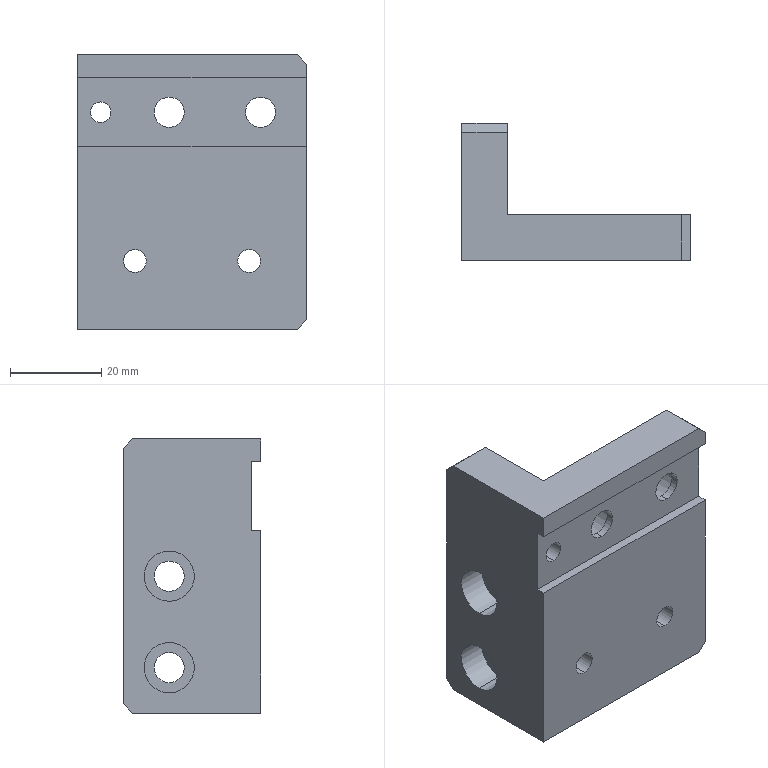Part | SolidWorks | features HoleWzd 4, Chamfer 1, Extrusion 1, ICE 1 | 1 solid | 45 faces | box 50 x 30 x 60 mm | volume 36632 mm3 | cylinder 24 | plane 21 | commonest cylinder face diameters 6.6 x8 11 x8 5 x4 4.5 x2 8 x2
STEP:
#1=CARTESIAN_POINT('',(12.5,10.,17.4));
#2=VERTEX_POINT('',#1);
#3=CARTESIAN_POINT('',(10.,10.,14.9));
#4=VERTEX_POINT('',#3);
#5=CARTESIAN_POINT('',(12.5,10.,14.9));
#6=DIRECTION('',(0.,-1.,0.));
#7=DIRECTION('',(0.,0.,-1.));
#8=AXIS2_PLACEMENT_3D('',#5,#6,#7);
#9=CIRCLE('',#8,2.5);
#10=EDGE_CURVE('',#2,#4,#9,.T.);
#11=ORIENTED_EDGE('',*,*,#10,.F.);
#12=CARTESIAN_POINT('',(12.5,0.,17.4));
#13=VERTEX_POINT('',#12);
#14=CARTESIAN_POINT('',(12.5,0.,17.4));
#15=DIRECTION('',(0.,-1.,0.));
#16=VECTOR('',#15,1000.);
#17=LINE('',#14,#16);
#18=EDGE_CURVE('',#2,#13,#17,.T.);
#19=ORIENTED_EDGE('',*,*,#18,.T.);
#20=CARTESIAN_POINT('',(12.5,0.,12.4));
#21=VERTEX_POINT('',#20);
#22=CARTESIAN_POINT('',(12.5,0.,14.9));
#23=DIRECTION('',(0.,-1.,0.));
#24=DIRECTION('',(0.,0.,-1.));
#25=AXIS2_PLACEMENT_3D('',#22,#23,#24);
#26=CIRCLE('',#25,2.5);
#27=EDGE_CURVE('',#13,#21,#26,.T.);
#28=ORIENTED_EDGE('',*,*,#27,.T.);
#29=CARTESIAN_POINT('',(12.5,10.,12.4));
#30=VERTEX_POINT('',#29);
#31=CARTESIAN_POINT('',(12.5,0.,12.4));
#32=DIRECTION('',(0.,-1.,0.));
#33=VECTOR('',#32,1000.);
#34=LINE('',#31,#33);
#35=EDGE_CURVE('',#30,#21,#34,.T.);
#36=ORIENTED_EDGE('',*,*,#35,.F.);
#37=CARTESIAN_POINT('',(12.5,10.,14.9));
#38=DIRECTION('',(0.,-1.,0.));
#39=DIRECTION('',(0.,0.,-1.));
#40=AXIS2_PLACEMENT_3D('',#37,#38,#39);
#41=CIRCLE('',#40,2.5);
#42=EDGE_CURVE('',#4,#30,#41,.T.);
#43=ORIENTED_EDGE('',*,*,#42,.F.);
#44=EDGE_LOOP('',(#11,#19,#28,#36,#43));
#45=FACE_OUTER_BOUND('',#44,.T.);
#46=CARTESIAN_POINT('',(12.5,0.,14.9));
#47=DIRECTION('',(0.,-1.,0.));
#48=DIRECTION('',(0.,0.,-1.));
#49=AXIS2_PLACEMENT_3D('',#46,#47,#48);
#50=CYLINDRICAL_SURFACE('',#49,2.5);
#51=ADVANCED_FACE('',(#45),#50,.F.);
#52=CARTESIAN_POINT('',(37.5,10.,17.4));
#53=VERTEX_POINT('',#52);
#54=CARTESIAN_POINT('',(37.5,10.,12.4));
#55=VERTEX_POINT('',#54);
#56=CARTESIAN_POINT('',(37.5,10.,14.9));
#57=DIRECTION('',(0.,-1.,0.));
#58=DIRECTION('',(0.,0.,-1.));
#59=AXIS2_PLACEMENT_3D('',#56,#57,#58);
#60=CIRCLE('',#59,2.5);
#61=EDGE_CURVE('',#53,#55,#60,.T.);
#62=ORIENTED_EDGE('',*,*,#61,.F.);
#63=CARTESIAN_POINT('',(37.5,0.,17.4));
#64=VERTEX_POINT('',#63);
#65=CARTESIAN_POINT('',(37.5,0.,17.4));
#66=DIRECTION('',(0.,-1.,0.));
#67=VECTOR('',#66,1000.);
#68=LINE('',#65,#67);
#69=EDGE_CURVE('',#53,#64,#68,.T.);
#70=ORIENTED_EDGE('',*,*,#69,.T.);
#71=CARTESIAN_POINT('',(37.5,0.,12.4));
#72=VERTEX_POINT('',#71);
#73=CARTESIAN_POINT('',(37.5,0.,14.9));
#74=DIRECTION('',(0.,-1.,0.));
#75=DIRECTION('',(0.,0.,-1.));
#76=AXIS2_PLACEMENT_3D('',#73,#74,#75);
#77=CIRCLE('',#76,2.5);
#78=EDGE_CURVE('',#64,#72,#77,.T.);
#79=ORIENTED_EDGE('',*,*,#78,.T.);
#80=CARTESIAN_POINT('',(37.5,0.,12.4));
#81=DIRECTION('',(0.,-1.,0.));
#82=VECTOR('',#81,1000.);
#83=LINE('',#80,#82);
#84=EDGE_CURVE('',#55,#72,#83,.T.);
#85=ORIENTED_EDGE('',*,*,#84,.F.);
#86=EDGE_LOOP('',(#62,#70,#79,#85));
#87=FACE_OUTER_BOUND('',#86,.T.);
#88=CARTESIAN_POINT('',(37.5,0.,14.9));
#89=DIRECTION('',(0.,-1.,0.));
#90=DIRECTION('',(0.,0.,-1.));
#91=AXIS2_PLACEMENT_3D('',#88,#89,#90);
#92=CYLINDRICAL_SURFACE('',#91,2.5);
#93=ADVANCED_FACE('',(#87),#92,.F.);
#94=CARTESIAN_POINT('',(6.4,20.,4.45));
#95=VERTEX_POINT('',#94);
#96=CARTESIAN_POINT('',(6.4,20.,15.45));
#97=VERTEX_POINT('',#96);
#98=CARTESIAN_POINT('',(6.4,20.,9.95));
#99=DIRECTION('',(-1.,0.,0.));
#100=DIRECTION('',(0.,0.,1.));
#101=AXIS2_PLACEMENT_3D('',#98,#99,#100);
#102=CIRCLE('',#101,5.5);
#103=EDGE_CURVE('',#95,#97,#102,.T.);
#104=ORIENTED_EDGE('',*,*,#103,.F.);
#105=CARTESIAN_POINT('',(0.,20.,4.45));
#106=VERTEX_POINT('',#105);
#107=CARTESIAN_POINT('',(0.,20.,4.45));
#108=DIRECTION('',(-1.,0.,0.));
#109=VECTOR('',#108,1000.);
#110=LINE('',#107,#109);
#111=EDGE_CURVE('',#95,#106,#110,.T.);
#112=ORIENTED_EDGE('',*,*,#111,.T.);
#113=CARTESIAN_POINT('',(0.,20.,15.45));
#114=VERTEX_POINT('',#113);
#115=CARTESIAN_POINT('',(0.,20.,9.95));
#116=DIRECTION('',(-1.,0.,0.));
#117=DIRECTION('',(0.,0.,1.));
#118=AXIS2_PLACEMENT_3D('',#115,#116,#117);
#119=CIRCLE('',#118,5.5);
#120=EDGE_CURVE('',#106,#114,#119,.T.);
#121=ORIENTED_EDGE('',*,*,#120,.T.);
#122=CARTESIAN_POINT('',(0.,20.,15.45));
#123=DIRECTION('',(-1.,0.,0.));
#124=VECTOR('',#123,1000.);
#125=LINE('',#122,#124);
#126=EDGE_CURVE('',#97,#114,#125,.T.);
#127=ORIENTED_EDGE('',*,*,#126,.F.);
#128=EDGE_LOOP('',(#104,#112,#121,#127));
#129=FACE_OUTER_BOUND('',#128,.T.);
#130=CARTESIAN_POINT('',(0.,20.,9.95));
#131=DIRECTION('',(-1.,0.,0.));
#132=DIRECTION('',(0.,0.,1.));
#133=AXIS2_PLACEMENT_3D('',#130,#131,#132);
#134=CYLINDRICAL_SURFACE('',#133,5.5);
#135=ADVANCED_FACE('',(#129),#134,.F.);
#136=CARTESIAN_POINT('',(10.,20.,6.65));
#137=VERTEX_POINT('',#136);
#138=CARTESIAN_POINT('',(10.,20.,13.25));
#139=VERTEX_POINT('',#138);
#140=CARTESIAN_POINT('',(10.,20.,9.95));
#141=DIRECTION('',(-1.,0.,0.));
#142=DIRECTION('',(0.,0.,1.));
#143=AXIS2_PLACEMENT_3D('',#140,#141,#142);
#144=CIRCLE('',#143,3.3);
#145=EDGE_CURVE('',#137,#139,#144,.T.);
#146=ORIENTED_EDGE('',*,*,#145,.F.);
#147=CARTESIAN_POINT('',(6.4,20.,6.65));
#148=VERTEX_POINT('',#147);
#149=CARTESIAN_POINT('',(0.,20.,6.65));
#150=DIRECTION('',(-1.,0.,0.));
#151=VECTOR('',#150,1000.);
#152=LINE('',#149,#151);
#153=EDGE_CURVE('',#137,#148,#152,.T.);
#154=ORIENTED_EDGE('',*,*,#153,.T.);
#155=CARTESIAN_POINT('',(6.4,20.,13.25));
#156=VERTEX_POINT('',#155);
#157=CARTESIAN_POINT('',(6.4,20.,9.95));
#158=DIRECTION('',(-1.,0.,0.));
#159=DIRECTION('',(0.,0.,1.));
#160=AXIS2_PLACEMENT_3D('',#157,#158,#159);
#161=CIRCLE('',#160,3.3);
#162=EDGE_CURVE('',#148,#156,#161,.T.);
#163=ORIENTED_EDGE('',*,*,#162,.T.);
#164=CARTESIAN_POINT('',(0.,20.,13.25));
#165=DIRECTION('',(-1.,0.,0.));
#166=VECTOR('',#165,1000.);
#167=LINE('',#164,#166);
#168=EDGE_CURVE('',#139,#156,#167,.T.);
#169=ORIENTED_EDGE('',*,*,#168,.F.);
#170=EDGE_LOOP('',(#146,#154,#163,#169));
#171=FACE_OUTER_BOUND('',#170,.T.);
#172=CARTESIAN_POINT('',(0.,20.,9.95));
#173=DIRECTION('',(-1.,0.,0.));
#174=DIRECTION('',(0.,0.,1.));
#175=AXIS2_PLACEMENT_3D('',#172,#173,#174);
#176=CYLINDRICAL_SURFACE('',#175,3.3);
#177=ADVANCED_FACE('',(#171),#176,.F.);
#178=CARTESIAN_POINT('',(6.4,20.,24.45));
#179=VERTEX_POINT('',#178);
#180=CARTESIAN_POINT('',(6.4,20.,35.45));
#181=VERTEX_POINT('',#180);
#182=CARTESIAN_POINT('',(6.4,20.,29.95));
#183=DIRECTION('',(-1.,0.,0.));
#184=DIRECTION('',(0.,0.,1.));
#185=AXIS2_PLACEMENT_3D('',#182,#183,#184);
#186=CIRCLE('',#185,5.5);
#187=EDGE_CURVE('',#179,#181,#186,.T.);
#188=ORIENTED_EDGE('',*,*,#187,.F.);
#189=CARTESIAN_POINT('',(0.,20.,24.45));
#190=VERTEX_POINT('',#189);
#191=CARTESIAN_POINT('',(0.,20.,24.45));
#192=DIRECTION('',(-1.,0.,0.));
#193=VECTOR('',#192,1000.);
#194=LINE('',#191,#193);
#195=EDGE_CURVE('',#179,#190,#194,.T.);
#196=ORIENTED_EDGE('',*,*,#195,.T.);
#197=CARTESIAN_POINT('',(0.,20.,35.45));
#198=VERTEX_POINT('',#197);
#199=CARTESIAN_POINT('',(0.,20.,29.95));
#200=DIRECTION('',(-1.,0.,0.));
#201=DIRECTION('',(0.,0.,1.));
#202=AXIS2_PLACEMENT_3D('',#199,#200,#201);
#203=CIRCLE('',#202,5.5);
#204=EDGE_CURVE('',#190,#198,#203,.T.);
#205=ORIENTED_EDGE('',*,*,#204,.T.);
#206=CARTESIAN_POINT('',(0.,20.,35.45));
#207=DIRECTION('',(-1.,0.,0.));
#208=VECTOR('',#207,1000.);
#209=LINE('',#206,#208);
#210=EDGE_CURVE('',#181,#198,#209,.T.);
#211=ORIENTED_EDGE('',*,*,#210,.F.);
#212=EDGE_LOOP('',(#188,#196,#205,#211));
#213=FACE_OUTER_BOUND('',#212,.T.);
#214=CARTESIAN_POINT('',(0.,20.,29.95));
#215=DIRECTION('',(-1.,0.,0.));
#216=DIRECTION('',(0.,0.,1.));
#217=AXIS2_PLACEMENT_3D('',#214,#215,#216);
#218=CYLINDRICAL_SURFACE('',#217,5.5);
#219=ADVANCED_FACE('',(#213),#218,.F.);
#220=CARTESIAN_POINT('',(10.,20.,26.65));
#221=VERTEX_POINT('',#220);
#222=CARTESIAN_POINT('',(10.,20.,33.25));
#223=VERTEX_POINT('',#222);
#224=CARTESIAN_POINT('',(10.,20.,29.95));
#225=DIRECTION('',(-1.,0.,0.));
#226=DIRECTION('',(0.,0.,1.));
#227=AXIS2_PLACEMENT_3D('',#224,#225,#226);
#228=CIRCLE('',#227,3.3);
#229=EDGE_CURVE('',#221,#223,#228,.T.);
#230=ORIENTED_EDGE('',*,*,#229,.F.);
#231=CARTESIAN_POINT('',(6.4,20.,26.65));
#232=VERTEX_POINT('',#231);
#233=CARTESIAN_POINT('',(0.,20.,26.65));
#234=DIRECTION('',(-1.,0.,0.));
#235=VECTOR('',#234,1000.);
#236=LINE('',#233,#235);
#237=EDGE_CURVE('',#221,#232,#236,.T.);
#238=ORIENTED_EDGE('',*,*,#237,.T.);
#239=CARTESIAN_POINT('',(6.4,20.,33.25));
#240=VERTEX_POINT('',#239);
#241=CARTESIAN_POINT('',(6.4,20.,29.95));
#242=DIRECTION('',(-1.,0.,0.));
#243=DIRECTION('',(0.,0.,1.));
#244=AXIS2_PLACEMENT_3D('',#241,#242,#243);
#245=CIRCLE('',#244,3.3);
#246=EDGE_CURVE('',#232,#240,#245,.T.);
#247=ORIENTED_EDGE('',*,*,#246,.T.);
#248=CARTESIAN_POINT('',(0.,20.,33.25));
#249=DIRECTION('',(-1.,0.,0.));
#250=VECTOR('',#249,1000.);
#251=LINE('',#248,#250);
#252=EDGE_CURVE('',#223,#240,#251,.T.);
#253=ORIENTED_EDGE('',*,*,#252,.F.);
#254=EDGE_LOOP('',(#230,#238,#247,#253));
#255=FACE_OUTER_BOUND('',#254,.T.);
#256=CARTESIAN_POINT('',(0.,20.,29.95));
#257=DIRECTION('',(-1.,0.,0.));
#258=DIRECTION('',(0.,0.,1.));
#259=AXIS2_PLACEMENT_3D('',#256,#257,#258);
#260=CYLINDRICAL_SURFACE('',#259,3.3);
#261=ADVANCED_FACE('',(#255),#260,.F.);
#262=CARTESIAN_POINT('',(20.,3.6,41.95));
#263=VERTEX_POINT('',#262);
#264=CARTESIAN_POINT('',(20.,3.6,52.95));
#265=VERTEX_POINT('',#264);
#266=CARTESIAN_POINT('',(20.,3.6,47.45));
#267=DIRECTION('',(0.,1.,0.));
#268=DIRECTION('',(0.,0.,1.));
#269=AXIS2_PLACEMENT_3D('',#266,#267,#268);
#270=CIRCLE('',#269,5.5);
#271=EDGE_CURVE('',#263,#265,#270,.T.);
#272=ORIENTED_EDGE('',*,*,#271,.F.);
#273=CARTESIAN_POINT('',(20.,10.,41.95));
#274=VERTEX_POINT('',#273);
#275=CARTESIAN_POINT('',(20.,10.,41.95));
#276=DIRECTION('',(0.,1.,0.));
#277=VECTOR('',#276,1000.);
#278=LINE('',#275,#277);
#279=EDGE_CURVE('',#263,#274,#278,.T.);
#280=ORIENTED_EDGE('',*,*,#279,.T.);
#281=CARTESIAN_POINT('',(20.,10.,52.95));
#282=VERTEX_POINT('',#281);
#283=CARTESIAN_POINT('',(20.,10.,47.45));
#284=DIRECTION('',(0.,1.,0.));
#285=DIRECTION('',(0.,0.,1.));
#286=AXIS2_PLACEMENT_3D('',#283,#284,#285);
#287=CIRCLE('',#286,5.5);
#288=EDGE_CURVE('',#274,#282,#287,.T.);
#289=ORIENTED_EDGE('',*,*,#288,.T.);
#290=CARTESIAN_POINT('',(20.,10.,52.95));
#291=DIRECTION('',(0.,1.,0.));
#292=VECTOR('',#291,1000.);
#293=LINE('',#290,#292);
#294=EDGE_CURVE('',#265,#282,#293,.T.);
#295=ORIENTED_EDGE('',*,*,#294,.F.);
#296=EDGE_LOOP('',(#272,#280,#289,#295));
#297=FACE_OUTER_BOUND('',#296,.T.);
#298=CARTESIAN_POINT('',(20.,10.,47.45));
#299=DIRECTION('',(0.,1.,0.));
#300=DIRECTION('',(0.,0.,1.));
#301=AXIS2_PLACEMENT_3D('',#298,#299,#300);
#302=CYLINDRICAL_SURFACE('',#301,5.5);
#303=ADVANCED_FACE('',(#297),#302,.F.);
#304=CARTESIAN_POINT('',(20.,2.,50.75));
#305=VERTEX_POINT('',#304);
#306=CARTESIAN_POINT('',(20.,2.,44.15));
#307=VERTEX_POINT('',#306);
#308=CARTESIAN_POINT('',(20.,2.,47.45));
#309=DIRECTION('',(0.,-1.,0.));
#310=DIRECTION('',(1.,0.,0.));
#311=AXIS2_PLACEMENT_3D('',#308,#309,#310);
#312=CIRCLE('',#311,3.3);
#313=EDGE_CURVE('',#305,#307,#312,.T.);
#314=ORIENTED_EDGE('',*,*,#313,.T.);
#315=CARTESIAN_POINT('',(20.,3.6,44.15));
#316=VERTEX_POINT('',#315);
#317=CARTESIAN_POINT('',(20.,10.,44.15));
#318=DIRECTION('',(0.,1.,0.));
#319=VECTOR('',#318,1000.);
#320=LINE('',#317,#319);
#321=EDGE_CURVE('',#307,#316,#320,.T.);
#322=ORIENTED_EDGE('',*,*,#321,.T.);
#323=CARTESIAN_POINT('',(20.,3.6,50.75));
#324=VERTEX_POINT('',#323);
#325=CARTESIAN_POINT('',(20.,3.6,47.45));
#326=DIRECTION('',(0.,1.,0.));
#327=DIRECTION('',(0.,0.,1.));
#328=AXIS2_PLACEMENT_3D('',#325,#326,#327);
#329=CIRCLE('',#328,3.3);
#330=EDGE_CURVE('',#316,#324,#329,.T.);
#331=ORIENTED_EDGE('',*,*,#330,.T.);
#332=CARTESIAN_POINT('',(20.,10.,50.75));
#333=DIRECTION('',(0.,1.,0.));
#334=VECTOR('',#333,1000.);
#335=LINE('',#332,#334);
#336=EDGE_CURVE('',#305,#324,#335,.T.);
#337=ORIENTED_EDGE('',*,*,#336,.F.);
#338=EDGE_LOOP('',(#314,#322,#331,#337));
#339=FACE_OUTER_BOUND('',#338,.T.);
#340=CARTESIAN_POINT('',(20.,10.,47.45));
#341=DIRECTION('',(0.,1.,0.));
#342=DIRECTION('',(0.,0.,1.));
#343=AXIS2_PLACEMENT_3D('',#340,#341,#342);
#344=CYLINDRICAL_SURFACE('',#343,3.3);
#345=ADVANCED_FACE('',(#339),#344,.F.);
#346=CARTESIAN_POINT('',(40.,3.6,41.95));
#347=VERTEX_POINT('',#346);
#348=CARTESIAN_POINT('',(40.,3.6,52.95));
#349=VERTEX_POINT('',#348);
#350=CARTESIAN_POINT('',(40.,3.6,47.45));
#351=DIRECTION('',(0.,1.,0.));
#352=DIRECTION('',(0.,0.,1.));
#353=AXIS2_PLACEMENT_3D('',#350,#351,#352);
#354=CIRCLE('',#353,5.5);
#355=EDGE_CURVE('',#347,#349,#354,.T.);
#356=ORIENTED_EDGE('',*,*,#355,.F.);
#357=CARTESIAN_POINT('',(40.,10.,41.95));
#358=VERTEX_POINT('',#357);
#359=CARTESIAN_POINT('',(40.,10.,41.95));
#360=DIRECTION('',(0.,1.,0.));
#361=VECTOR('',#360,1000.);
#362=LINE('',#359,#361);
#363=EDGE_CURVE('',#347,#358,#362,.T.);
#364=ORIENTED_EDGE('',*,*,#363,.T.);
#365=CARTESIAN_POINT('',(40.,10.,52.95));
#366=VERTEX_POINT('',#365);
#367=CARTESIAN_POINT('',(40.,10.,47.45));
#368=DIRECTION('',(0.,1.,0.));
#369=DIRECTION('',(0.,0.,1.));
#370=AXIS2_PLACEMENT_3D('',#367,#368,#369);
#371=CIRCLE('',#370,5.5);
#372=EDGE_CURVE('',#358,#366,#371,.T.);
#373=ORIENTED_EDGE('',*,*,#372,.T.);
#374=CARTESIAN_POINT('',(40.,10.,52.95));
#375=DIRECTION('',(0.,1.,0.));
#376=VECTOR('',#375,1000.);
#377=LINE('',#374,#376);
#378=EDGE_CURVE('',#349,#366,#377,.T.);
#379=ORIENTED_EDGE('',*,*,#378,.F.);
#380=EDGE_LOOP('',(#356,#364,#373,#379));
#381=FACE_OUTER_BOUND('',#380,.T.);
#382=CARTESIAN_POINT('',(40.,10.,47.45));
#383=DIRECTION('',(0.,1.,0.));
#384=DIRECTION('',(0.,0.,1.));
#385=AXIS2_PLACEMENT_3D('',#382,#383,#384);
#386=CYLINDRICAL_SURFACE('',#385,5.5);
#387=ADVANCED_FACE('',(#381),#386,.F.);
#388=CARTESIAN_POINT('',(40.,2.,50.75));
#389=VERTEX_POINT('',#388);
#390=CARTESIAN_POINT('',(40.,2.,44.15));
#391=VERTEX_POINT('',#390);
#392=CARTESIAN_POINT('',(40.,2.,47.45));
#393=DIRECTION('',(0.,-1.,0.));
#394=DIRECTION('',(1.,0.,0.));
#395=AXIS2_PLACEMENT_3D('',#392,#393,#394);
#396=CIRCLE('',#395,3.3);
#397=EDGE_CURVE('',#389,#391,#396,.T.);
#398=ORIENTED_EDGE('',*,*,#397,.T.);
#399=CARTESIAN_POINT('',(40.,3.6,44.15));
#400=VERTEX_POINT('',#399);
#401=CARTESIAN_POINT('',(40.,10.,44.15));
#402=DIRECTION('',(0.,1.,0.));
#403=VECTOR('',#402,1000.);
#404=LINE('',#401,#403);
#405=EDGE_CURVE('',#391,#400,#404,.T.);
#406=ORIENTED_EDGE('',*,*,#405,.T.);
#407=CARTESIAN_POINT('',(40.,3.6,50.75));
#408=VERTEX_POINT('',#407);
#409=CARTESIAN_POINT('',(40.,3.6,47.45));
#410=DIRECTION('',(0.,1.,0.));
#411=DIRECTION('',(0.,0.,1.));
#412=AXIS2_PLACEMENT_3D('',#409,#410,#411);
#413=CIRCLE('',#412,3.3);
#414=EDGE_CURVE('',#400,#408,#413,.T.);
#415=ORIENTED_EDGE('',*,*,#414,.T.);
#416=CARTESIAN_POINT('',(40.,10.,50.75));
#417=DIRECTION('',(0.,1.,0.));
#418=VECTOR('',#417,1000.);
#419=LINE('',#416,#418);
#420=EDGE_CURVE('',#389,#408,#419,.T.);
#421=ORIENTED_EDGE('',*,*,#420,.F.);
#422=EDGE_LOOP('',(#398,#406,#415,#421));
#423=FACE_OUTER_BOUND('',#422,.T.);
#424=CARTESIAN_POINT('',(40.,10.,47.45));
#425=DIRECTION('',(0.,1.,0.));
#426=DIRECTION('',(0.,0.,1.));
#427=AXIS2_PLACEMENT_3D('',#424,#425,#426);
#428=CYLINDRICAL_SURFACE('',#427,3.3);
#429=ADVANCED_FACE('',(#423),#428,.F.);
#430=CARTESIAN_POINT('',(5.,25.6,43.45));
#431=VERTEX_POINT('',#430);
#432=CARTESIAN_POINT('',(5.,25.6,51.45));
#433=VERTEX_POINT('',#432);
#434=CARTESIAN_POINT('',(5.,25.6,47.45));
#435=DIRECTION('',(0.,1.,0.));
#436=DIRECTION('',(0.,0.,1.));
#437=AXIS2_PLACEMENT_3D('',#434,#435,#436);
#438=CIRCLE('',#437,4.);
#439=EDGE_CURVE('',#431,#433,#438,.T.);
#440=ORIENTED_EDGE('',*,*,#439,.F.);
#441=CARTESIAN_POINT('',(5.,30.,43.45));
#442=VERTEX_POINT('',#441);
#443=CARTESIAN_POINT('',(5.,30.,43.45));
#444=DIRECTION('',(0.,1.,0.));
#445=VECTOR('',#444,1000.);
#446=LINE('',#443,#445);
#447=EDGE_CURVE('',#431,#442,#446,.T.);
#448=ORIENTED_EDGE('',*,*,#447,.T.);
#449=CARTESIAN_POINT('',(5.,30.,51.45));
#450=VERTEX_POINT('',#449);
#451=CARTESIAN_POINT('',(5.,30.,47.45));
#452=DIRECTION('',(0.,1.,0.));
#453=DIRECTION('',(0.,0.,1.));
#454=AXIS2_PLACEMENT_3D('',#451,#452,#453);
#455=CIRCLE('',#454,4.);
#456=EDGE_CURVE('',#442,#450,#455,.T.);
#457=ORIENTED_EDGE('',*,*,#456,.T.);
#458=CARTESIAN_POINT('',(5.,30.,51.45));
#459=DIRECTION('',(0.,1.,0.));
#460=VECTOR('',#459,1000.);
#461=LINE('',#458,#460);
#462=EDGE_CURVE('',#433,#450,#461,.T.);
#463=ORIENTED_EDGE('',*,*,#462,.F.);
#464=EDGE_LOOP('',(#440,#448,#457,#463));
#465=FACE_OUTER_BOUND('',#464,.T.);
#466=CARTESIAN_POINT('',(5.,30.,47.45));
#467=DIRECTION('',(0.,1.,0.));
#468=DIRECTION('',(0.,0.,1.));
#469=AXIS2_PLACEMENT_3D('',#466,#467,#468);
#470=CYLINDRICAL_SURFACE('',#469,4.);
#471=ADVANCED_FACE('',(#465),#470,.F.);
#472=CARTESIAN_POINT('',(5.,2.,49.7));
#473=VERTEX_POINT('',#472);
#474=CARTESIAN_POINT('',(5.,2.,45.2));
#475=VERTEX_POINT('',#474);
#476=CARTESIAN_POINT('',(5.,2.,47.45));
#477=DIRECTION('',(0.,-1.,0.));
#478=DIRECTION('',(1.,0.,0.));
#479=AXIS2_PLACEMENT_3D('',#476,#477,#478);
#480=CIRCLE('',#479,2.25);
#481=EDGE_CURVE('',#473,#475,#480,.T.);
#482=ORIENTED_EDGE('',*,*,#481,.T.);
#483=CARTESIAN_POINT('',(5.,25.6,45.2));
#484=VERTEX_POINT('',#483);
#485=CARTESIAN_POINT('',(5.,30.,45.2));
#486=DIRECTION('',(0.,1.,0.));
#487=VECTOR('',#486,1000.);
#488=LINE('',#485,#487);
#489=EDGE_CURVE('',#475,#484,#488,.T.);
#490=ORIENTED_EDGE('',*,*,#489,.T.);
#491=CARTESIAN_POINT('',(5.,25.6,49.7));
#492=VERTEX_POINT('',#491);
#493=CARTESIAN_POINT('',(5.,25.6,47.45));
#494=DIRECTION('',(0.,1.,0.));
#495=DIRECTION('',(0.,0.,1.));
#496=AXIS2_PLACEMENT_3D('',#493,#494,#495);
#497=CIRCLE('',#496,2.25);
#498=EDGE_CURVE('',#484,#492,#497,.T.);
#499=ORIENTED_EDGE('',*,*,#498,.T.);
#500=CARTESIAN_POINT('',(5.,30.,49.7));
#501=DIRECTION('',(0.,1.,0.));
#502=VECTOR('',#501,1000.);
#503=LINE('',#500,#502);
#504=EDGE_CURVE('',#473,#492,#503,.T.);
#505=ORIENTED_EDGE('',*,*,#504,.F.);
#506=EDGE_LOOP('',(#482,#490,#499,#505));
#507=FACE_OUTER_BOUND('',#506,.T.);
#508=CARTESIAN_POINT('',(5.,30.,47.45));
#509=DIRECTION('',(0.,1.,0.));
#510=DIRECTION('',(0.,0.,1.));
#511=AXIS2_PLACEMENT_3D('',#508,#509,#510);
#512=CYLINDRICAL_SURFACE('',#511,2.25);
#513=ADVANCED_FACE('',(#507),#512,.F.);
#514=CARTESIAN_POINT('',(50.,0.,58.));
#515=VERTEX_POINT('',#514);
#516=CARTESIAN_POINT('',(50.,0.,55.));
#517=VERTEX_POINT('',#516);
#518=CARTESIAN_POINT('',(50.,0.,60.));
#519=DIRECTION('',(0.,0.,-1.));
#520=VECTOR('',#519,1000.);
#521=LINE('',#518,#520);
#522=EDGE_CURVE('',#515,#517,#521,.T.);
#523=ORIENTED_EDGE('',*,*,#522,.F.);
#524=CARTESIAN_POINT('',(48.,0.,60.));
#525=VERTEX_POINT('',#524);
#526=CARTESIAN_POINT('',(48.,0.,60.));
#527=DIRECTION('',(-0.7071,0.,0.7071));
#528=VECTOR('',#527,1000.);
#529=LINE('',#526,#528);
#530=EDGE_CURVE('',#515,#525,#529,.T.);
#531=ORIENTED_EDGE('',*,*,#530,.T.);
#532=CARTESIAN_POINT('',(0.,0.,60.));
#533=VERTEX_POINT('',#532);
#534=CARTESIAN_POINT('',(50.,0.,60.));
#535=DIRECTION('',(1.,0.,0.));
#536=VECTOR('',#535,1000.);
#537=LINE('',#534,#536);
#538=EDGE_CURVE('',#533,#525,#537,.T.);
#539=ORIENTED_EDGE('',*,*,#538,.F.);
#540=CARTESIAN_POINT('',(0.,0.,55.));
#541=VERTEX_POINT('',#540);
#542=CARTESIAN_POINT('',(0.,0.,60.));
#543=DIRECTION('',(0.,0.,-1.));
#544=VECTOR('',#543,1000.);
#545=LINE('',#542,#544);
#546=EDGE_CURVE('',#533,#541,#545,.T.);
#547=ORIENTED_EDGE('',*,*,#546,.T.);
#548=CARTESIAN_POINT('',(0.,0.,55.));
#549=DIRECTION('',(-1.,0.,0.));
#550=VECTOR('',#549,1000.);
#551=LINE('',#548,#550);
#552=EDGE_CURVE('',#517,#541,#551,.T.);
#553=ORIENTED_EDGE('',*,*,#552,.F.);
#554=EDGE_LOOP('',(#523,#531,#539,#547,#553));
#555=FACE_OUTER_BOUND('',#554,.T.);
#556=CARTESIAN_POINT('',(50.,0.,60.));
#557=DIRECTION('',(0.,1.,0.));
#558=DIRECTION('',(-1.,0.,0.));
#559=AXIS2_PLACEMENT_3D('',#556,#557,#558);
#560=PLANE('',#559);
#561=ADVANCED_FACE('',(#555),#560,.F.);
#562=CARTESIAN_POINT('',(50.,10.,58.));
#563=VERTEX_POINT('',#562);
#564=CARTESIAN_POINT('',(50.,10.,2.));
#565=VERTEX_POINT('',#564);
#566=CARTESIAN_POINT('',(50.,10.,60.));
#567=DIRECTION('',(0.,0.,-1.));
#568=VECTOR('',#567,1000.);
#569=LINE('',#566,#568);
#570=EDGE_CURVE('',#563,#565,#569,.T.);
#571=ORIENTED_EDGE('',*,*,#570,.F.);
#572=CARTESIAN_POINT('',(50.,10.,58.));
#573=DIRECTION('',(0.,-1.,0.));
#574=VECTOR('',#573,1000.);
#575=LINE('',#572,#574);
#576=EDGE_CURVE('',#563,#515,#575,.T.);
#577=ORIENTED_EDGE('',*,*,#576,.T.);
#578=ORIENTED_EDGE('',*,*,#522,.T.);
#579=CARTESIAN_POINT('',(50.,2.,55.));
#580=VERTEX_POINT('',#579);
#581=CARTESIAN_POINT('',(50.,2.,55.));
#582=DIRECTION('',(0.,-1.,0.));
#583=VECTOR('',#582,1000.);
#584=LINE('',#581,#583);
#585=EDGE_CURVE('',#580,#517,#584,.T.);
#586=ORIENTED_EDGE('',*,*,#585,.F.);
#587=CARTESIAN_POINT('',(50.,2.,39.9));
#588=VERTEX_POINT('',#587);
#589=CARTESIAN_POINT('',(50.,2.,55.));
#590=DIRECTION('',(0.,0.,1.));
#591=VECTOR('',#590,1000.);
#592=LINE('',#589,#591);
#593=EDGE_CURVE('',#588,#580,#592,.T.);
#594=ORIENTED_EDGE('',*,*,#593,.F.);
#595=CARTESIAN_POINT('',(50.,0.,39.9));
#596=VERTEX_POINT('',#595);
#597=CARTESIAN_POINT('',(50.,2.,39.9));
#598=DIRECTION('',(0.,-1.,0.));
#599=VECTOR('',#598,1000.);
#600=LINE('',#597,#599);
#601=EDGE_CURVE('',#588,#596,#600,.T.);
#602=ORIENTED_EDGE('',*,*,#601,.T.);
#603=CARTESIAN_POINT('',(50.,0.,2.));
#604=VERTEX_POINT('',#603);
#605=CARTESIAN_POINT('',(50.,0.,60.));
#606=DIRECTION('',(0.,0.,-1.));
#607=VECTOR('',#606,1000.);
#608=LINE('',#605,#607);
#609=EDGE_CURVE('',#596,#604,#608,.T.);
#610=ORIENTED_EDGE('',*,*,#609,.T.);
#611=CARTESIAN_POINT('',(50.,10.,2.));
#612=DIRECTION('',(0.,1.,0.));
#613=VECTOR('',#612,1000.);
#614=LINE('',#611,#613);
#615=EDGE_CURVE('',#604,#565,#614,.T.);
#616=ORIENTED_EDGE('',*,*,#615,.T.);
#617=EDGE_LOOP('',(#571,#577,#578,#586,#594,#602,#610,#616));
#618=FACE_OUTER_BOUND('',#617,.T.);
#619=CARTESIAN_POINT('',(50.,10.,60.));
#620=DIRECTION('',(-1.,0.,0.));
#621=DIRECTION('',(0.,0.,1.));
#622=AXIS2_PLACEMENT_3D('',#619,#620,#621);
#623=PLANE('',#622);
#624=ADVANCED_FACE('',(#618),#623,.F.);
#625=CARTESIAN_POINT('',(37.5,10.,14.9));
#626=DIRECTION('',(0.,-1.,0.));
#627=DIRECTION('',(0.,0.,-1.));
#628=AXIS2_PLACEMENT_3D('',#625,#626,#627);
#629=CIRCLE('',#628,2.5);
#630=EDGE_CURVE('',#55,#53,#629,.T.);
#631=ORIENTED_EDGE('',*,*,#630,.T.);
#632=ORIENTED_EDGE('',*,*,#61,.T.);
#633=EDGE_LOOP('',(#631,#632));
#634=FACE_BOUND('',#633,.T.);
#635=CARTESIAN_POINT('',(20.,10.,47.45));
#636=DIRECTION('',(0.,1.,0.));
#637=DIRECTION('',(0.,0.,1.));
#638=AXIS2_PLACEMENT_3D('',#635,#636,#637);
#639=CIRCLE('',#638,5.5);
#640=EDGE_CURVE('',#282,#274,#639,.T.);
#641=ORIENTED_EDGE('',*,*,#640,.F.);
#642=ORIENTED_EDGE('',*,*,#288,.F.);
#643=EDGE_LOOP('',(#641,#642));
#644=FACE_BOUND('',#643,.T.);
#645=CARTESIAN_POINT('',(40.,10.,47.45));
#646=DIRECTION('',(0.,1.,0.));
#647=DIRECTION('',(0.,0.,1.));
#648=AXIS2_PLACEMENT_3D('',#645,#646,#647);
#649=CIRCLE('',#648,5.5);
#650=EDGE_CURVE('',#366,#358,#649,.T.);
#651=ORIENTED_EDGE('',*,*,#650,.F.);
#652=ORIENTED_EDGE('',*,*,#372,.F.);
#653=EDGE_LOOP('',(#651,#652));
#654=FACE_BOUND('',#653,.T.);
#655=CARTESIAN_POINT('',(10.,10.,0.));
#656=VERTEX_POINT('',#655);
#657=CARTESIAN_POINT('',(10.,10.,60.));
#658=DIRECTION('',(0.,0.,-1.));
#659=VECTOR('',#658,1000.);
#660=LINE('',#657,#659);
#661=EDGE_CURVE('',#4,#656,#660,.T.);
#662=ORIENTED_EDGE('',*,*,#661,.F.);
#663=ORIENTED_EDGE('',*,*,#42,.T.);
#664=CARTESIAN_POINT('',(12.5,10.,14.9));
#665=DIRECTION('',(0.,-1.,0.));
#666=DIRECTION('',(0.,0.,-1.));
#667=AXIS2_PLACEMENT_3D('',#664,#665,#666);
#668=CIRCLE('',#667,2.5);
#669=EDGE_CURVE('',#30,#2,#668,.T.);
#670=ORIENTED_EDGE('',*,*,#669,.T.);
#671=ORIENTED_EDGE('',*,*,#10,.T.);
#672=CARTESIAN_POINT('',(10.,10.,60.));
#673=VERTEX_POINT('',#672);
#674=CARTESIAN_POINT('',(10.,10.,60.));
#675=DIRECTION('',(0.,0.,-1.));
#676=VECTOR('',#675,1000.);
#677=LINE('',#674,#676);
#678=EDGE_CURVE('',#673,#4,#677,.T.);
#679=ORIENTED_EDGE('',*,*,#678,.F.);
#680=CARTESIAN_POINT('',(48.,10.,60.));
#681=VERTEX_POINT('',#680);
#682=CARTESIAN_POINT('',(50.,10.,60.));
#683=DIRECTION('',(-1.,0.,0.));
#684=VECTOR('',#683,1000.);
#685=LINE('',#682,#684);
#686=EDGE_CURVE('',#681,#673,#685,.T.);
#687=ORIENTED_EDGE('',*,*,#686,.F.);
#688=CARTESIAN_POINT('',(48.,10.,60.));
#689=DIRECTION('',(0.7071,0.,-0.7071));
#690=VECTOR('',#689,1000.);
#691=LINE('',#688,#690);
#692=EDGE_CURVE('',#681,#563,#691,.T.);
#693=ORIENTED_EDGE('',*,*,#692,.T.);
#694=ORIENTED_EDGE('',*,*,#570,.T.);
#695=CARTESIAN_POINT('',(48.,10.,0.));
#696=VERTEX_POINT('',#695);
#697=CARTESIAN_POINT('',(50.,10.,2.));
#698=DIRECTION('',(-0.7071,0.,-0.7071));
#699=VECTOR('',#698,1000.);
#700=LINE('',#697,#699);
#701=EDGE_CURVE('',#565,#696,#700,.T.);
#702=ORIENTED_EDGE('',*,*,#701,.T.);
#703=CARTESIAN_POINT('',(50.,10.,0.));
#704=DIRECTION('',(-1.,0.,0.));
#705=VECTOR('',#704,1000.);
#706=LINE('',#703,#705);
#707=EDGE_CURVE('',#696,#656,#706,.T.);
#708=ORIENTED_EDGE('',*,*,#707,.T.);
#709=EDGE_LOOP('',(#662,#663,#670,#671,#679,#687,#693,#694,#702,#708));
#710=FACE_OUTER_BOUND('',#709,.T.);
#711=CARTESIAN_POINT('',(50.,10.,60.));
#712=DIRECTION('',(0.,-1.,0.));
#713=DIRECTION('',(0.,0.,-1.));
#714=AXIS2_PLACEMENT_3D('',#711,#712,#713);
#715=PLANE('',#714);
#716=ADVANCED_FACE('',(#634,#644,#654,#710),#715,.F.);
#717=ORIENTED_EDGE('',*,*,#678,.T.);
#718=ORIENTED_EDGE('',*,*,#661,.T.);
#719=CARTESIAN_POINT('',(10.,28.,0.));
#720=VERTEX_POINT('',#719);
#721=CARTESIAN_POINT('',(10.,10.,0.));
#722=DIRECTION('',(0.,1.,0.));
#723=VECTOR('',#722,1000.);
#724=LINE('',#721,#723);
#725=EDGE_CURVE('',#656,#720,#724,.T.);
#726=ORIENTED_EDGE('',*,*,#725,.T.);
#727=CARTESIAN_POINT('',(10.,30.,2.));
#728=VERTEX_POINT('',#727);
#729=CARTESIAN_POINT('',(10.,30.,2.));
#730=DIRECTION('',(0.,0.7071,0.7071));
#731=VECTOR('',#730,1000.);
#732=LINE('',#729,#731);
#733=EDGE_CURVE('',#720,#728,#732,.T.);
#734=ORIENTED_EDGE('',*,*,#733,.T.);
#735=CARTESIAN_POINT('',(10.,30.,58.));
#736=VERTEX_POINT('',#735);
#737=CARTESIAN_POINT('',(10.,30.,60.));
#738=DIRECTION('',(0.,0.,-1.));
#739=VECTOR('',#738,1000.);
#740=LINE('',#737,#739);
#741=EDGE_CURVE('',#736,#728,#740,.T.);
#742=ORIENTED_EDGE('',*,*,#741,.F.);
#743=CARTESIAN_POINT('',(10.,28.,60.));
#744=VERTEX_POINT('',#743);
#745=CARTESIAN_POINT('',(10.,28.,60.));
#746=DIRECTION('',(0.,-0.7071,0.7071));
#747=VECTOR('',#746,1000.);
#748=LINE('',#745,#747);
#749=EDGE_CURVE('',#736,#744,#748,.T.);
#750=ORIENTED_EDGE('',*,*,#749,.T.);
#751=CARTESIAN_POINT('',(10.,10.,60.));
#752=DIRECTION('',(0.,1.,0.));
#753=VECTOR('',#752,1000.);
#754=LINE('',#751,#753);
#755=EDGE_CURVE('',#673,#744,#754,.T.);
#756=ORIENTED_EDGE('',*,*,#755,.F.);
#757=EDGE_LOOP('',(#717,#718,#726,#734,#742,#750,#756));
#758=FACE_OUTER_BOUND('',#757,.T.);
#759=CARTESIAN_POINT('',(10.,20.,9.95));
#760=DIRECTION('',(-1.,0.,0.));
#761=DIRECTION('',(0.,0.,1.));
#762=AXIS2_PLACEMENT_3D('',#759,#760,#761);
#763=CIRCLE('',#762,3.3);
#764=EDGE_CURVE('',#139,#137,#763,.T.);
#765=ORIENTED_EDGE('',*,*,#764,.T.);
#766=ORIENTED_EDGE('',*,*,#145,.T.);
#767=EDGE_LOOP('',(#765,#766));
#768=FACE_BOUND('',#767,.T.);
#769=CARTESIAN_POINT('',(10.,20.,29.95));
#770=DIRECTION('',(-1.,0.,0.));
#771=DIRECTION('',(0.,0.,1.));
#772=AXIS2_PLACEMENT_3D('',#769,#770,#771);
#773=CIRCLE('',#772,3.3);
#774=EDGE_CURVE('',#223,#221,#773,.T.);
#775=ORIENTED_EDGE('',*,*,#774,.T.);
#776=ORIENTED_EDGE('',*,*,#229,.T.);
#777=EDGE_LOOP('',(#775,#776));
#778=FACE_BOUND('',#777,.T.);
#779=CARTESIAN_POINT('',(10.,10.,60.));
#780=DIRECTION('',(-1.,0.,0.));
#781=DIRECTION('',(0.,0.,1.));
#782=AXIS2_PLACEMENT_3D('',#779,#780,#781);
#783=PLANE('',#782);
#784=ADVANCED_FACE('',(#758,#768,#778),#783,.F.);
#785=CARTESIAN_POINT('',(5.,30.,47.45));
#786=DIRECTION('',(0.,1.,0.));
#787=DIRECTION('',(0.,0.,1.));
#788=AXIS2_PLACEMENT_3D('',#785,#786,#787);
#789=CIRCLE('',#788,4.);
#790=EDGE_CURVE('',#450,#442,#789,.T.);
#791=ORIENTED_EDGE('',*,*,#790,.F.);
#792=ORIENTED_EDGE('',*,*,#456,.F.);
#793=EDGE_LOOP('',(#791,#792));
#794=FACE_BOUND('',#793,.T.);
#795=ORIENTED_EDGE('',*,*,#741,.T.);
#796=CARTESIAN_POINT('',(0.,30.,2.));
#797=VERTEX_POINT('',#796);
#798=CARTESIAN_POINT('',(0.,30.,2.));
#799=DIRECTION('',(-1.,0.,0.));
#800=VECTOR('',#799,1000.);
#801=LINE('',#798,#800);
#802=EDGE_CURVE('',#728,#797,#801,.T.);
#803=ORIENTED_EDGE('',*,*,#802,.T.);
#804=CARTESIAN_POINT('',(0.,30.,58.));
#805=VERTEX_POINT('',#804);
#806=CARTESIAN_POINT('',(0.,30.,60.));
#807=DIRECTION('',(0.,0.,-1.));
#808=VECTOR('',#807,1000.);
#809=LINE('',#806,#808);
#810=EDGE_CURVE('',#805,#797,#809,.T.);
#811=ORIENTED_EDGE('',*,*,#810,.F.);
#812=CARTESIAN_POINT('',(10.,30.,58.));
#813=DIRECTION('',(1.,0.,0.));
#814=VECTOR('',#813,1000.);
#815=LINE('',#812,#814);
#816=EDGE_CURVE('',#805,#736,#815,.T.);
#817=ORIENTED_EDGE('',*,*,#816,.T.);
#818=EDGE_LOOP('',(#795,#803,#811,#817));
#819=FACE_OUTER_BOUND('',#818,.T.);
#820=CARTESIAN_POINT('',(10.,30.,60.));
#821=DIRECTION('',(0.,-1.,0.));
#822=DIRECTION('',(0.,0.,-1.));
#823=AXIS2_PLACEMENT_3D('',#820,#821,#822);
#824=PLANE('',#823);
#825=ADVANCED_FACE('',(#794,#819),#824,.F.);
#826=CARTESIAN_POINT('',(0.,20.,9.95));
#827=DIRECTION('',(-1.,0.,0.));
#828=DIRECTION('',(0.,0.,1.));
#829=AXIS2_PLACEMENT_3D('',#826,#827,#828);
#830=CIRCLE('',#829,5.5);
#831=EDGE_CURVE('',#114,#106,#830,.T.);
#832=ORIENTED_EDGE('',*,*,#831,.F.);
#833=ORIENTED_EDGE('',*,*,#120,.F.);
#834=EDGE_LOOP('',(#832,#833));
#835=FACE_BOUND('',#834,.T.);
#836=CARTESIAN_POINT('',(0.,20.,29.95));
#837=DIRECTION('',(-1.,0.,0.));
#838=DIRECTION('',(0.,0.,1.));
#839=AXIS2_PLACEMENT_3D('',#836,#837,#838);
#840=CIRCLE('',#839,5.5);
#841=EDGE_CURVE('',#198,#190,#840,.T.);
#842=ORIENTED_EDGE('',*,*,#841,.F.);
#843=ORIENTED_EDGE('',*,*,#204,.F.);
#844=EDGE_LOOP('',(#842,#843));
#845=FACE_BOUND('',#844,.T.);
#846=ORIENTED_EDGE('',*,*,#810,.T.);
#847=CARTESIAN_POINT('',(0.,28.,0.));
#848=VERTEX_POINT('',#847);
#849=CARTESIAN_POINT('',(0.,30.,2.));
#850=DIRECTION('',(0.,-0.7071,-0.7071));
#851=VECTOR('',#850,1000.);
#852=LINE('',#849,#851);
#853=EDGE_CURVE('',#797,#848,#852,.T.);
#854=ORIENTED_EDGE('',*,*,#853,.T.);
#855=CARTESIAN_POINT('',(0.,0.,0.));
#856=VERTEX_POINT('',#855);
#857=CARTESIAN_POINT('',(0.,0.,0.));
#858=DIRECTION('',(0.,-1.,0.));
#859=VECTOR('',#858,1000.);
#860=LINE('',#857,#859);
#861=EDGE_CURVE('',#848,#856,#860,.T.);
#862=ORIENTED_EDGE('',*,*,#861,.T.);
#863=CARTESIAN_POINT('',(0.,0.,39.9));
#864=VERTEX_POINT('',#863);
#865=CARTESIAN_POINT('',(0.,0.,60.));
#866=DIRECTION('',(0.,0.,-1.));
#867=VECTOR('',#866,1000.);
#868=LINE('',#865,#867);
#869=EDGE_CURVE('',#864,#856,#868,.T.);
#870=ORIENTED_EDGE('',*,*,#869,.F.);
#871=CARTESIAN_POINT('',(0.,2.,39.9));
#872=VERTEX_POINT('',#871);
#873=CARTESIAN_POINT('',(0.,2.,39.9));
#874=DIRECTION('',(0.,-1.,0.));
#875=VECTOR('',#874,1000.);
#876=LINE('',#873,#875);
#877=EDGE_CURVE('',#872,#864,#876,.T.);
#878=ORIENTED_EDGE('',*,*,#877,.F.);
#879=CARTESIAN_POINT('',(0.,2.,55.));
#880=VERTEX_POINT('',#879);
#881=CARTESIAN_POINT('',(0.,2.,55.));
#882=DIRECTION('',(0.,0.,-1.));
#883=VECTOR('',#882,1000.);
#884=LINE('',#881,#883);
#885=EDGE_CURVE('',#880,#872,#884,.T.);
#886=ORIENTED_EDGE('',*,*,#885,.F.);
#887=CARTESIAN_POINT('',(0.,2.,55.));
#888=DIRECTION('',(0.,-1.,0.));
#889=VECTOR('',#888,1000.);
#890=LINE('',#887,#889);
#891=EDGE_CURVE('',#880,#541,#890,.T.);
#892=ORIENTED_EDGE('',*,*,#891,.T.);
#893=ORIENTED_EDGE('',*,*,#546,.F.);
#894=CARTESIAN_POINT('',(0.,28.,60.));
#895=VERTEX_POINT('',#894);
#896=CARTESIAN_POINT('',(0.,0.,60.));
#897=DIRECTION('',(0.,-1.,0.));
#898=VECTOR('',#897,1000.);
#899=LINE('',#896,#898);
#900=EDGE_CURVE('',#895,#533,#899,.T.);
#901=ORIENTED_EDGE('',*,*,#900,.F.);
#902=CARTESIAN_POINT('',(0.,28.,60.));
#903=DIRECTION('',(0.,0.7071,-0.7071));
#904=VECTOR('',#903,1000.);
#905=LINE('',#902,#904);
#906=EDGE_CURVE('',#895,#805,#905,.T.);
#907=ORIENTED_EDGE('',*,*,#906,.T.);
#908=EDGE_LOOP('',(#846,#854,#862,#870,#878,#886,#892,#893,#901,#907));
#909=FACE_OUTER_BOUND('',#908,.T.);
#910=CARTESIAN_POINT('',(0.,0.,60.));
#911=DIRECTION('',(1.,0.,0.));
#912=DIRECTION('',(0.,1.,0.));
#913=AXIS2_PLACEMENT_3D('',#910,#911,#912);
#914=PLANE('',#913);
#915=ADVANCED_FACE('',(#835,#845,#909),#914,.F.);
#916=CARTESIAN_POINT('',(12.5,0.,14.9));
#917=DIRECTION('',(0.,-1.,0.));
#918=DIRECTION('',(0.,0.,-1.));
#919=AXIS2_PLACEMENT_3D('',#916,#917,#918);
#920=CIRCLE('',#919,2.5);
#921=EDGE_CURVE('',#21,#13,#920,.T.);
#922=ORIENTED_EDGE('',*,*,#921,.F.);
#923=ORIENTED_EDGE('',*,*,#27,.F.);
#924=EDGE_LOOP('',(#922,#923));
#925=FACE_BOUND('',#924,.T.);
#926=CARTESIAN_POINT('',(37.5,0.,14.9));
#927=DIRECTION('',(0.,-1.,0.));
#928=DIRECTION('',(0.,0.,-1.));
#929=AXIS2_PLACEMENT_3D('',#926,#927,#928);
#930=CIRCLE('',#929,2.5);
#931=EDGE_CURVE('',#72,#64,#930,.T.);
#932=ORIENTED_EDGE('',*,*,#931,.F.);
#933=ORIENTED_EDGE('',*,*,#78,.F.);
#934=EDGE_LOOP('',(#932,#933));
#935=FACE_BOUND('',#934,.T.);
#936=CARTESIAN_POINT('',(48.,0.,0.));
#937=VERTEX_POINT('',#936);
#938=CARTESIAN_POINT('',(50.,0.,0.));
#939=DIRECTION('',(1.,0.,0.));
#940=VECTOR('',#939,1000.);
#941=LINE('',#938,#940);
#942=EDGE_CURVE('',#856,#937,#941,.T.);
#943=ORIENTED_EDGE('',*,*,#942,.T.);
#944=CARTESIAN_POINT('',(50.,0.,2.));
#945=DIRECTION('',(0.7071,0.,0.7071));
#946=VECTOR('',#945,1000.);
#947=LINE('',#944,#946);
#948=EDGE_CURVE('',#937,#604,#947,.T.);
#949=ORIENTED_EDGE('',*,*,#948,.T.);
#950=ORIENTED_EDGE('',*,*,#609,.F.);
#951=CARTESIAN_POINT('',(0.,0.,39.9));
#952=DIRECTION('',(1.,0.,0.));
#953=VECTOR('',#952,1000.);
#954=LINE('',#951,#953);
#955=EDGE_CURVE('',#864,#596,#954,.T.);
#956=ORIENTED_EDGE('',*,*,#955,.F.);
#957=ORIENTED_EDGE('',*,*,#869,.T.);
#958=EDGE_LOOP('',(#943,#949,#950,#956,#957));
#959=FACE_OUTER_BOUND('',#958,.T.);
#960=CARTESIAN_POINT('',(50.,0.,60.));
#961=DIRECTION('',(0.,1.,0.));
#962=DIRECTION('',(-1.,0.,0.));
#963=AXIS2_PLACEMENT_3D('',#960,#961,#962);
#964=PLANE('',#963);
#965=ADVANCED_FACE('',(#925,#935,#959),#964,.F.);
#966=ORIENTED_EDGE('',*,*,#538,.T.);
#967=CARTESIAN_POINT('',(48.,0.,60.));
#968=DIRECTION('',(0.,1.,0.));
#969=VECTOR('',#968,1000.);
#970=LINE('',#967,#969);
#971=EDGE_CURVE('',#525,#681,#970,.T.);
#972=ORIENTED_EDGE('',*,*,#971,.T.);
#973=ORIENTED_EDGE('',*,*,#686,.T.);
#974=ORIENTED_EDGE('',*,*,#755,.T.);
#975=CARTESIAN_POINT('',(0.,28.,60.));
#976=DIRECTION('',(-1.,0.,0.));
#977=VECTOR('',#976,1000.);
#978=LINE('',#975,#977);
#979=EDGE_CURVE('',#744,#895,#978,.T.);
#980=ORIENTED_EDGE('',*,*,#979,.T.);
#981=ORIENTED_EDGE('',*,*,#900,.T.);
#982=EDGE_LOOP('',(#966,#972,#973,#974,#980,#981));
#983=FACE_OUTER_BOUND('',#982,.T.);
#984=CARTESIAN_POINT('',(0.,0.,60.));
#985=DIRECTION('',(0.,0.,-1.));
#986=DIRECTION('',(-1.,0.,0.));
#987=AXIS2_PLACEMENT_3D('',#984,#985,#986);
#988=PLANE('',#987);
#989=ADVANCED_FACE('',(#983),#988,.F.);
#990=ORIENTED_EDGE('',*,*,#707,.F.);
#991=CARTESIAN_POINT('',(48.,0.,0.));
#992=DIRECTION('',(0.,-1.,0.));
#993=VECTOR('',#992,1000.);
#994=LINE('',#991,#993);
#995=EDGE_CURVE('',#696,#937,#994,.T.);
#996=ORIENTED_EDGE('',*,*,#995,.T.);
#997=ORIENTED_EDGE('',*,*,#942,.F.);
#998=ORIENTED_EDGE('',*,*,#861,.F.);
#999=CARTESIAN_POINT('',(10.,28.,0.));
#1000=DIRECTION('',(1.,0.,0.));
#1001=VECTOR('',#1000,1000.);
#1002=LINE('',#999,#1001);
#1003=EDGE_CURVE('',#848,#720,#1002,.T.);
#1004=ORIENTED_EDGE('',*,*,#1003,.T.);
#1005=ORIENTED_EDGE('',*,*,#725,.F.);
#1006=EDGE_LOOP('',(#990,#996,#997,#998,#1004,#1005));
#1007=FACE_OUTER_BOUND('',#1006,.T.);
#1008=CARTESIAN_POINT('',(0.,0.,0.));
#1009=DIRECTION('',(0.,0.,-1.));
#1010=DIRECTION('',(-1.,0.,0.));
#1011=AXIS2_PLACEMENT_3D('',#1008,#1009,#1010);
#1012=PLANE('',#1011);
#1013=ADVANCED_FACE('',(#1007),#1012,.T.);
#1014=ORIENTED_EDGE('',*,*,#552,.T.);
#1015=ORIENTED_EDGE('',*,*,#891,.F.);
#1016=CARTESIAN_POINT('',(0.,2.,55.));
#1017=DIRECTION('',(-1.,0.,0.));
#1018=VECTOR('',#1017,1000.);
#1019=LINE('',#1016,#1018);
#1020=EDGE_CURVE('',#580,#880,#1019,.T.);
#1021=ORIENTED_EDGE('',*,*,#1020,.F.);
#1022=ORIENTED_EDGE('',*,*,#585,.T.);
#1023=EDGE_LOOP('',(#1014,#1015,#1021,#1022));
#1024=FACE_OUTER_BOUND('',#1023,.T.);
#1025=CARTESIAN_POINT('',(0.,2.,55.));
#1026=DIRECTION('',(0.,0.,1.));
#1027=DIRECTION('',(1.,0.,0.));
#1028=AXIS2_PLACEMENT_3D('',#1025,#1026,#1027);
#1029=PLANE('',#1028);
#1030=ADVANCED_FACE('',(#1024),#1029,.F.);
#1031=ORIENTED_EDGE('',*,*,#955,.T.);
#1032=ORIENTED_EDGE('',*,*,#601,.F.);
#1033=CARTESIAN_POINT('',(0.,2.,39.9));
#1034=DIRECTION('',(1.,0.,0.));
#1035=VECTOR('',#1034,1000.);
#1036=LINE('',#1033,#1035);
#1037=EDGE_CURVE('',#872,#588,#1036,.T.);
#1038=ORIENTED_EDGE('',*,*,#1037,.F.);
#1039=ORIENTED_EDGE('',*,*,#877,.T.);
#1040=EDGE_LOOP('',(#1031,#1032,#1038,#1039));
#1041=FACE_OUTER_BOUND('',#1040,.T.);
#1042=CARTESIAN_POINT('',(0.,2.,39.9));
#1043=DIRECTION('',(0.,0.,-1.));
#1044=DIRECTION('',(-1.,0.,0.));
#1045=AXIS2_PLACEMENT_3D('',#1042,#1043,#1044);
#1046=PLANE('',#1045);
#1047=ADVANCED_FACE('',(#1041),#1046,.F.);
#1048=ORIENTED_EDGE('',*,*,#313,.F.);
#1049=CARTESIAN_POINT('',(20.,2.,47.45));
#1050=DIRECTION('',(0.,-1.,0.));
#1051=DIRECTION('',(1.,0.,0.));
#1052=AXIS2_PLACEMENT_3D('',#1049,#1050,#1051);
#1053=CIRCLE('',#1052,3.3);
#1054=EDGE_CURVE('',#307,#305,#1053,.T.);
#1055=ORIENTED_EDGE('',*,*,#1054,.F.);
#1056=EDGE_LOOP('',(#1048,#1055));
#1057=FACE_BOUND('',#1056,.T.);
#1058=ORIENTED_EDGE('',*,*,#397,.F.);
#1059=CARTESIAN_POINT('',(40.,2.,47.45));
#1060=DIRECTION('',(0.,-1.,0.));
#1061=DIRECTION('',(1.,0.,0.));
#1062=AXIS2_PLACEMENT_3D('',#1059,#1060,#1061);
#1063=CIRCLE('',#1062,3.3);
#1064=EDGE_CURVE('',#391,#389,#1063,.T.);
#1065=ORIENTED_EDGE('',*,*,#1064,.F.);
#1066=EDGE_LOOP('',(#1058,#1065));
#1067=FACE_BOUND('',#1066,.T.);
#1068=ORIENTED_EDGE('',*,*,#481,.F.);
#1069=CARTESIAN_POINT('',(5.,2.,47.45));
#1070=DIRECTION('',(0.,-1.,0.));
#1071=DIRECTION('',(1.,0.,0.));
#1072=AXIS2_PLACEMENT_3D('',#1069,#1070,#1071);
#1073=CIRCLE('',#1072,2.25);
#1074=EDGE_CURVE('',#475,#473,#1073,.T.);
#1075=ORIENTED_EDGE('',*,*,#1074,.F.);
#1076=EDGE_LOOP('',(#1068,#1075));
#1077=FACE_BOUND('',#1076,.T.);
#1078=ORIENTED_EDGE('',*,*,#885,.T.);
#1079=ORIENTED_EDGE('',*,*,#1037,.T.);
#1080=ORIENTED_EDGE('',*,*,#593,.T.);
#1081=ORIENTED_EDGE('',*,*,#1020,.T.);
#1082=EDGE_LOOP('',(#1078,#1079,#1080,#1081));
#1083=FACE_OUTER_BOUND('',#1082,.T.);
#1084=CARTESIAN_POINT('',(0.,2.,0.));
#1085=DIRECTION('',(0.,-1.,0.));
#1086=DIRECTION('',(1.,0.,0.));
#1087=AXIS2_PLACEMENT_3D('',#1084,#1085,#1086);
#1088=PLANE('',#1087);
#1089=ADVANCED_FACE('',(#1057,#1067,#1077,#1083),#1088,.T.);
#1090=ORIENTED_EDGE('',*,*,#489,.F.);
#1091=ORIENTED_EDGE('',*,*,#1074,.T.);
#1092=ORIENTED_EDGE('',*,*,#504,.T.);
#1093=CARTESIAN_POINT('',(5.,25.6,47.45));
#1094=DIRECTION('',(0.,1.,0.));
#1095=DIRECTION('',(0.,0.,1.));
#1096=AXIS2_PLACEMENT_3D('',#1093,#1094,#1095);
#1097=CIRCLE('',#1096,2.25);
#1098=EDGE_CURVE('',#492,#484,#1097,.T.);
#1099=ORIENTED_EDGE('',*,*,#1098,.T.);
#1100=EDGE_LOOP('',(#1090,#1091,#1092,#1099));
#1101=FACE_OUTER_BOUND('',#1100,.T.);
#1102=CARTESIAN_POINT('',(5.,30.,47.45));
#1103=DIRECTION('',(0.,1.,0.));
#1104=DIRECTION('',(0.,0.,1.));
#1105=AXIS2_PLACEMENT_3D('',#1102,#1103,#1104);
#1106=CYLINDRICAL_SURFACE('',#1105,2.25);
#1107=ADVANCED_FACE('',(#1101),#1106,.F.);
#1108=ORIENTED_EDGE('',*,*,#1098,.F.);
#1109=ORIENTED_EDGE('',*,*,#498,.F.);
#1110=EDGE_LOOP('',(#1108,#1109));
#1111=FACE_BOUND('',#1110,.T.);
#1112=CARTESIAN_POINT('',(5.,25.6,47.45));
#1113=DIRECTION('',(0.,1.,0.));
#1114=DIRECTION('',(0.,0.,1.));
#1115=AXIS2_PLACEMENT_3D('',#1112,#1113,#1114);
#1116=CIRCLE('',#1115,4.);
#1117=EDGE_CURVE('',#433,#431,#1116,.T.);
#1118=ORIENTED_EDGE('',*,*,#1117,.T.);
#1119=ORIENTED_EDGE('',*,*,#439,.T.);
#1120=EDGE_LOOP('',(#1118,#1119));
#1121=FACE_OUTER_BOUND('',#1120,.T.);
#1122=CARTESIAN_POINT('',(7.25,25.6,47.45));
#1123=DIRECTION('',(0.,-1.,0.));
#1124=DIRECTION('',(0.,0.,-1.));
#1125=AXIS2_PLACEMENT_3D('',#1122,#1123,#1124);
#1126=PLANE('',#1125);
#1127=ADVANCED_FACE('',(#1111,#1121),#1126,.F.);
#1128=ORIENTED_EDGE('',*,*,#447,.F.);
#1129=ORIENTED_EDGE('',*,*,#1117,.F.);
#1130=ORIENTED_EDGE('',*,*,#462,.T.);
#1131=ORIENTED_EDGE('',*,*,#790,.T.);
#1132=EDGE_LOOP('',(#1128,#1129,#1130,#1131));
#1133=FACE_OUTER_BOUND('',#1132,.T.);
#1134=CARTESIAN_POINT('',(5.,30.,47.45));
#1135=DIRECTION('',(0.,1.,0.));
#1136=DIRECTION('',(0.,0.,1.));
#1137=AXIS2_PLACEMENT_3D('',#1134,#1135,#1136);
#1138=CYLINDRICAL_SURFACE('',#1137,4.);
#1139=ADVANCED_FACE('',(#1133),#1138,.F.);
#1140=ORIENTED_EDGE('',*,*,#405,.F.);
#1141=ORIENTED_EDGE('',*,*,#1064,.T.);
#1142=ORIENTED_EDGE('',*,*,#420,.T.);
#1143=CARTESIAN_POINT('',(40.,3.6,47.45));
#1144=DIRECTION('',(0.,1.,0.));
#1145=DIRECTION('',(0.,0.,1.));
#1146=AXIS2_PLACEMENT_3D('',#1143,#1144,#1145);
#1147=CIRCLE('',#1146,3.3);
#1148=EDGE_CURVE('',#408,#400,#1147,.T.);
#1149=ORIENTED_EDGE('',*,*,#1148,.T.);
#1150=EDGE_LOOP('',(#1140,#1141,#1142,#1149));
#1151=FACE_OUTER_BOUND('',#1150,.T.);
#1152=CARTESIAN_POINT('',(40.,10.,47.45));
#1153=DIRECTION('',(0.,1.,0.));
#1154=DIRECTION('',(0.,0.,1.));
#1155=AXIS2_PLACEMENT_3D('',#1152,#1153,#1154);
#1156=CYLINDRICAL_SURFACE('',#1155,3.3);
#1157=ADVANCED_FACE('',(#1151),#1156,.F.);
#1158=ORIENTED_EDGE('',*,*,#1148,.F.);
#1159=ORIENTED_EDGE('',*,*,#414,.F.);
#1160=EDGE_LOOP('',(#1158,#1159));
#1161=FACE_BOUND('',#1160,.T.);
#1162=CARTESIAN_POINT('',(40.,3.6,47.45));
#1163=DIRECTION('',(0.,1.,0.));
#1164=DIRECTION('',(0.,0.,1.));
#1165=AXIS2_PLACEMENT_3D('',#1162,#1163,#1164);
#1166=CIRCLE('',#1165,5.5);
#1167=EDGE_CURVE('',#349,#347,#1166,.T.);
#1168=ORIENTED_EDGE('',*,*,#1167,.T.);
#1169=ORIENTED_EDGE('',*,*,#355,.T.);
#1170=EDGE_LOOP('',(#1168,#1169));
#1171=FACE_OUTER_BOUND('',#1170,.T.);
#1172=CARTESIAN_POINT('',(43.3,3.6,47.45));
#1173=DIRECTION('',(0.,-1.,0.));
#1174=DIRECTION('',(0.,0.,-1.));
#1175=AXIS2_PLACEMENT_3D('',#1172,#1173,#1174);
#1176=PLANE('',#1175);
#1177=ADVANCED_FACE('',(#1161,#1171),#1176,.F.);
#1178=ORIENTED_EDGE('',*,*,#363,.F.);
#1179=ORIENTED_EDGE('',*,*,#1167,.F.);
#1180=ORIENTED_EDGE('',*,*,#378,.T.);
#1181=ORIENTED_EDGE('',*,*,#650,.T.);
#1182=EDGE_LOOP('',(#1178,#1179,#1180,#1181));
#1183=FACE_OUTER_BOUND('',#1182,.T.);
#1184=CARTESIAN_POINT('',(40.,10.,47.45));
#1185=DIRECTION('',(0.,1.,0.));
#1186=DIRECTION('',(0.,0.,1.));
#1187=AXIS2_PLACEMENT_3D('',#1184,#1185,#1186);
#1188=CYLINDRICAL_SURFACE('',#1187,5.5);
#1189=ADVANCED_FACE('',(#1183),#1188,.F.);
#1190=ORIENTED_EDGE('',*,*,#321,.F.);
#1191=ORIENTED_EDGE('',*,*,#1054,.T.);
#1192=ORIENTED_EDGE('',*,*,#336,.T.);
#1193=CARTESIAN_POINT('',(20.,3.6,47.45));
#1194=DIRECTION('',(0.,1.,0.));
#1195=DIRECTION('',(0.,0.,1.));
#1196=AXIS2_PLACEMENT_3D('',#1193,#1194,#1195);
#1197=CIRCLE('',#1196,3.3);
#1198=EDGE_CURVE('',#324,#316,#1197,.T.);
#1199=ORIENTED_EDGE('',*,*,#1198,.T.);
#1200=EDGE_LOOP('',(#1190,#1191,#1192,#1199));
#1201=FACE_OUTER_BOUND('',#1200,.T.);
#1202=CARTESIAN_POINT('',(20.,10.,47.45));
#1203=DIRECTION('',(0.,1.,0.));
#1204=DIRECTION('',(0.,0.,1.));
#1205=AXIS2_PLACEMENT_3D('',#1202,#1203,#1204);
#1206=CYLINDRICAL_SURFACE('',#1205,3.3);
#1207=ADVANCED_FACE('',(#1201),#1206,.F.);
#1208=ORIENTED_EDGE('',*,*,#1198,.F.);
#1209=ORIENTED_EDGE('',*,*,#330,.F.);
#1210=EDGE_LOOP('',(#1208,#1209));
#1211=FACE_BOUND('',#1210,.T.);
#1212=CARTESIAN_POINT('',(20.,3.6,47.45));
#1213=DIRECTION('',(0.,1.,0.));
#1214=DIRECTION('',(0.,0.,1.));
#1215=AXIS2_PLACEMENT_3D('',#1212,#1213,#1214);
#1216=CIRCLE('',#1215,5.5);
#1217=EDGE_CURVE('',#265,#263,#1216,.T.);
#1218=ORIENTED_EDGE('',*,*,#1217,.T.);
#1219=ORIENTED_EDGE('',*,*,#271,.T.);
#1220=EDGE_LOOP('',(#1218,#1219));
#1221=FACE_OUTER_BOUND('',#1220,.T.);
#1222=CARTESIAN_POINT('',(23.3,3.6,47.45));
#1223=DIRECTION('',(0.,-1.,0.));
#1224=DIRECTION('',(0.,0.,-1.));
#1225=AXIS2_PLACEMENT_3D('',#1222,#1223,#1224);
#1226=PLANE('',#1225);
#1227=ADVANCED_FACE('',(#1211,#1221),#1226,.F.);
#1228=ORIENTED_EDGE('',*,*,#279,.F.);
#1229=ORIENTED_EDGE('',*,*,#1217,.F.);
#1230=ORIENTED_EDGE('',*,*,#294,.T.);
#1231=ORIENTED_EDGE('',*,*,#640,.T.);
#1232=EDGE_LOOP('',(#1228,#1229,#1230,#1231));
#1233=FACE_OUTER_BOUND('',#1232,.T.);
#1234=CARTESIAN_POINT('',(20.,10.,47.45));
#1235=DIRECTION('',(0.,1.,0.));
#1236=DIRECTION('',(0.,0.,1.));
#1237=AXIS2_PLACEMENT_3D('',#1234,#1235,#1236);
#1238=CYLINDRICAL_SURFACE('',#1237,5.5);
#1239=ADVANCED_FACE('',(#1233),#1238,.F.);
#1240=ORIENTED_EDGE('',*,*,#237,.F.);
#1241=ORIENTED_EDGE('',*,*,#774,.F.);
#1242=ORIENTED_EDGE('',*,*,#252,.T.);
#1243=CARTESIAN_POINT('',(6.4,20.,29.95));
#1244=DIRECTION('',(-1.,0.,0.));
#1245=DIRECTION('',(0.,0.,1.));
#1246=AXIS2_PLACEMENT_3D('',#1243,#1244,#1245);
#1247=CIRCLE('',#1246,3.3);
#1248=EDGE_CURVE('',#240,#232,#1247,.T.);
#1249=ORIENTED_EDGE('',*,*,#1248,.T.);
#1250=EDGE_LOOP('',(#1240,#1241,#1242,#1249));
#1251=FACE_OUTER_BOUND('',#1250,.T.);
#1252=CARTESIAN_POINT('',(0.,20.,29.95));
#1253=DIRECTION('',(-1.,0.,0.));
#1254=DIRECTION('',(0.,0.,1.));
#1255=AXIS2_PLACEMENT_3D('',#1252,#1253,#1254);
#1256=CYLINDRICAL_SURFACE('',#1255,3.3);
#1257=ADVANCED_FACE('',(#1251),#1256,.F.);
#1258=ORIENTED_EDGE('',*,*,#1248,.F.);
#1259=ORIENTED_EDGE('',*,*,#246,.F.);
#1260=EDGE_LOOP('',(#1258,#1259));
#1261=FACE_BOUND('',#1260,.T.);
#1262=CARTESIAN_POINT('',(6.4,20.,29.95));
#1263=DIRECTION('',(-1.,0.,0.));
#1264=DIRECTION('',(0.,0.,1.));
#1265=AXIS2_PLACEMENT_3D('',#1262,#1263,#1264);
#1266=CIRCLE('',#1265,5.5);
#1267=EDGE_CURVE('',#181,#179,#1266,.T.);
#1268=ORIENTED_EDGE('',*,*,#1267,.T.);
#1269=ORIENTED_EDGE('',*,*,#187,.T.);
#1270=EDGE_LOOP('',(#1268,#1269));
#1271=FACE_OUTER_BOUND('',#1270,.T.);
#1272=CARTESIAN_POINT('',(6.4,23.3,29.95));
#1273=DIRECTION('',(1.,0.,0.));
#1274=DIRECTION('',(0.,0.,-1.));
#1275=AXIS2_PLACEMENT_3D('',#1272,#1273,#1274);
#1276=PLANE('',#1275);
#1277=ADVANCED_FACE('',(#1261,#1271),#1276,.F.);
#1278=ORIENTED_EDGE('',*,*,#195,.F.);
#1279=ORIENTED_EDGE('',*,*,#1267,.F.);
#1280=ORIENTED_EDGE('',*,*,#210,.T.);
#1281=ORIENTED_EDGE('',*,*,#841,.T.);
#1282=EDGE_LOOP('',(#1278,#1279,#1280,#1281));
#1283=FACE_OUTER_BOUND('',#1282,.T.);
#1284=CARTESIAN_POINT('',(0.,20.,29.95));
#1285=DIRECTION('',(-1.,0.,0.));
#1286=DIRECTION('',(0.,0.,1.));
#1287=AXIS2_PLACEMENT_3D('',#1284,#1285,#1286);
#1288=CYLINDRICAL_SURFACE('',#1287,5.5);
#1289=ADVANCED_FACE('',(#1283),#1288,.F.);
#1290=ORIENTED_EDGE('',*,*,#153,.F.);
#1291=ORIENTED_EDGE('',*,*,#764,.F.);
#1292=ORIENTED_EDGE('',*,*,#168,.T.);
#1293=CARTESIAN_POINT('',(6.4,20.,9.95));
#1294=DIRECTION('',(-1.,0.,0.));
#1295=DIRECTION('',(0.,0.,1.));
#1296=AXIS2_PLACEMENT_3D('',#1293,#1294,#1295);
#1297=CIRCLE('',#1296,3.3);
#1298=EDGE_CURVE('',#156,#148,#1297,.T.);
#1299=ORIENTED_EDGE('',*,*,#1298,.T.);
#1300=EDGE_LOOP('',(#1290,#1291,#1292,#1299));
#1301=FACE_OUTER_BOUND('',#1300,.T.);
#1302=CARTESIAN_POINT('',(0.,20.,9.95));
#1303=DIRECTION('',(-1.,0.,0.));
#1304=DIRECTION('',(0.,0.,1.));
#1305=AXIS2_PLACEMENT_3D('',#1302,#1303,#1304);
#1306=CYLINDRICAL_SURFACE('',#1305,3.3);
#1307=ADVANCED_FACE('',(#1301),#1306,.F.);
#1308=ORIENTED_EDGE('',*,*,#1298,.F.);
#1309=ORIENTED_EDGE('',*,*,#162,.F.);
#1310=EDGE_LOOP('',(#1308,#1309));
#1311=FACE_BOUND('',#1310,.T.);
#1312=CARTESIAN_POINT('',(6.4,20.,9.95));
#1313=DIRECTION('',(-1.,0.,0.));
#1314=DIRECTION('',(0.,0.,1.));
#1315=AXIS2_PLACEMENT_3D('',#1312,#1313,#1314);
#1316=CIRCLE('',#1315,5.5);
#1317=EDGE_CURVE('',#97,#95,#1316,.T.);
#1318=ORIENTED_EDGE('',*,*,#1317,.T.);
#1319=ORIENTED_EDGE('',*,*,#103,.T.);
#1320=EDGE_LOOP('',(#1318,#1319));
#1321=FACE_OUTER_BOUND('',#1320,.T.);
#1322=CARTESIAN_POINT('',(6.4,23.3,9.95));
#1323=DIRECTION('',(1.,0.,0.));
#1324=DIRECTION('',(0.,0.,-1.));
#1325=AXIS2_PLACEMENT_3D('',#1322,#1323,#1324);
#1326=PLANE('',#1325);
#1327=ADVANCED_FACE('',(#1311,#1321),#1326,.F.);
#1328=ORIENTED_EDGE('',*,*,#111,.F.);
#1329=ORIENTED_EDGE('',*,*,#1317,.F.);
#1330=ORIENTED_EDGE('',*,*,#126,.T.);
#1331=ORIENTED_EDGE('',*,*,#831,.T.);
#1332=EDGE_LOOP('',(#1328,#1329,#1330,#1331));
#1333=FACE_OUTER_BOUND('',#1332,.T.);
#1334=CARTESIAN_POINT('',(0.,20.,9.95));
#1335=DIRECTION('',(-1.,0.,0.));
#1336=DIRECTION('',(0.,0.,1.));
#1337=AXIS2_PLACEMENT_3D('',#1334,#1335,#1336);
#1338=CYLINDRICAL_SURFACE('',#1337,5.5);
#1339=ADVANCED_FACE('',(#1333),#1338,.F.);
#1340=ORIENTED_EDGE('',*,*,#530,.F.);
#1341=ORIENTED_EDGE('',*,*,#576,.F.);
#1342=ORIENTED_EDGE('',*,*,#692,.F.);
#1343=ORIENTED_EDGE('',*,*,#971,.F.);
#1344=EDGE_LOOP('',(#1340,#1341,#1342,#1343));
#1345=FACE_OUTER_BOUND('',#1344,.T.);
#1346=CARTESIAN_POINT('',(48.,0.,60.));
#1347=DIRECTION('',(-0.7071,0.,-0.7071));
#1348=DIRECTION('',(0.,1.,0.));
#1349=AXIS2_PLACEMENT_3D('',#1346,#1347,#1348);
#1350=PLANE('',#1349);
#1351=ADVANCED_FACE('',(#1345),#1350,.F.);
#1352=ORIENTED_EDGE('',*,*,#948,.F.);
#1353=ORIENTED_EDGE('',*,*,#995,.F.);
#1354=ORIENTED_EDGE('',*,*,#701,.F.);
#1355=ORIENTED_EDGE('',*,*,#615,.F.);
#1356=EDGE_LOOP('',(#1352,#1353,#1354,#1355));
#1357=FACE_OUTER_BOUND('',#1356,.T.);
#1358=CARTESIAN_POINT('',(50.,10.,2.));
#1359=DIRECTION('',(0.7071,0.,-0.7071));
#1360=DIRECTION('',(0.,-1.,0.));
#1361=AXIS2_PLACEMENT_3D('',#1358,#1359,#1360);
#1362=PLANE('',#1361);
#1363=ADVANCED_FACE('',(#1357),#1362,.T.);
#1364=ORIENTED_EDGE('',*,*,#733,.F.);
#1365=ORIENTED_EDGE('',*,*,#1003,.F.);
#1366=ORIENTED_EDGE('',*,*,#853,.F.);
#1367=ORIENTED_EDGE('',*,*,#802,.F.);
#1368=EDGE_LOOP('',(#1364,#1365,#1366,#1367));
#1369=FACE_OUTER_BOUND('',#1368,.T.);
#1370=CARTESIAN_POINT('',(10.,30.,2.));
#1371=DIRECTION('',(0.,0.7071,-0.7071));
#1372=DIRECTION('',(1.,0.,0.));
#1373=AXIS2_PLACEMENT_3D('',#1370,#1371,#1372);
#1374=PLANE('',#1373);
#1375=ADVANCED_FACE('',(#1369),#1374,.T.);
#1376=ORIENTED_EDGE('',*,*,#749,.F.);
#1377=ORIENTED_EDGE('',*,*,#816,.F.);
#1378=ORIENTED_EDGE('',*,*,#906,.F.);
#1379=ORIENTED_EDGE('',*,*,#979,.F.);
#1380=EDGE_LOOP('',(#1376,#1377,#1378,#1379));
#1381=FACE_OUTER_BOUND('',#1380,.T.);
#1382=CARTESIAN_POINT('',(0.,28.,60.));
#1383=DIRECTION('',(0.,-0.7071,-0.7071));
#1384=DIRECTION('',(-1.,0.,0.));
#1385=AXIS2_PLACEMENT_3D('',#1382,#1383,#1384);
#1386=PLANE('',#1385);
#1387=ADVANCED_FACE('',(#1381),#1386,.F.);
#1388=ORIENTED_EDGE('',*,*,#69,.F.);
#1389=ORIENTED_EDGE('',*,*,#630,.F.);
#1390=ORIENTED_EDGE('',*,*,#84,.T.);
#1391=ORIENTED_EDGE('',*,*,#931,.T.);
#1392=EDGE_LOOP('',(#1388,#1389,#1390,#1391));
#1393=FACE_OUTER_BOUND('',#1392,.T.);
#1394=CARTESIAN_POINT('',(37.5,0.,14.9));
#1395=DIRECTION('',(0.,-1.,0.));
#1396=DIRECTION('',(0.,0.,-1.));
#1397=AXIS2_PLACEMENT_3D('',#1394,#1395,#1396);
#1398=CYLINDRICAL_SURFACE('',#1397,2.5);
#1399=ADVANCED_FACE('',(#1393),#1398,.F.);
#1400=ORIENTED_EDGE('',*,*,#18,.F.);
#1401=ORIENTED_EDGE('',*,*,#669,.F.);
#1402=ORIENTED_EDGE('',*,*,#35,.T.);
#1403=ORIENTED_EDGE('',*,*,#921,.T.);
#1404=EDGE_LOOP('',(#1400,#1401,#1402,#1403));
#1405=FACE_OUTER_BOUND('',#1404,.T.);
#1406=CARTESIAN_POINT('',(12.5,0.,14.9));
#1407=DIRECTION('',(0.,-1.,0.));
#1408=DIRECTION('',(0.,0.,-1.));
#1409=AXIS2_PLACEMENT_3D('',#1406,#1407,#1408);
#1410=CYLINDRICAL_SURFACE('',#1409,2.5);
#1411=ADVANCED_FACE('',(#1405),#1410,.F.);
#1412=CLOSED_SHELL('',(#51,#93,#135,#177,#219,#261,#303,#345,#387,#429,#471,#513,#561,#624,#716,#784,#825,#915,#965,#989,#1013,#1030,#1047,#1089,#1107,#1127,#1139,#1157,#1177,#1189,#1207,#1227,#1239,#1257,#1277,#1289,#1307,#1327,#1339,#1351,#1363,#1375,#1387,#1399,#1411));
#1413=MANIFOLD_SOLID_BREP('',#1412);
#1414=CARTESIAN_POINT('',(0.,0.,0.));
#1415=DIRECTION('',(0.,0.,1.));
#1416=DIRECTION('',(1.,0.,0.));
#1417=AXIS2_PLACEMENT_3D('',#1414,#1415,#1416);
#1418=(LENGTH_UNIT()NAMED_UNIT(*)SI_UNIT(.MILLI.,.METRE.));
#1419=UNCERTAINTY_MEASURE_WITH_UNIT(LENGTH_MEASURE(0.00001),#1418,'','');
#1420=(NAMED_UNIT(*)PLANE_ANGLE_UNIT()SI_UNIT($,.RADIAN.));
#1421=(NAMED_UNIT(*)SI_UNIT($,.STERADIAN.)SOLID_ANGLE_UNIT());
#1422=(GEOMETRIC_REPRESENTATION_CONTEXT(3)GLOBAL_UNCERTAINTY_ASSIGNED_CONTEXT((#1419))GLOBAL_UNIT_ASSIGNED_CONTEXT((#1418,#1420,#1421))REPRESENTATION_CONTEXT('',''));
#1423=ADVANCED_BREP_SHAPE_REPRESENTATION('',(#1413,#1417),#1422);